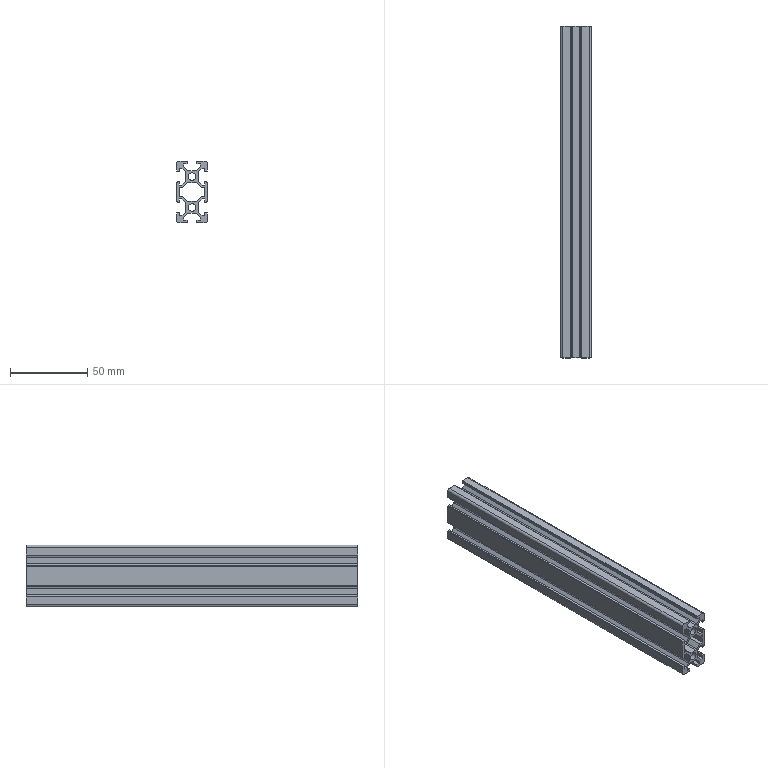Part | STEP file | YBQDJ-SSJ-5 | 1 solid | 124 faces | box 20 x 215 x 40 mm | volume 63524 mm3 | plane 102 | cylinder 22 | commonest cylinder face diameters 3 x20 5 x2